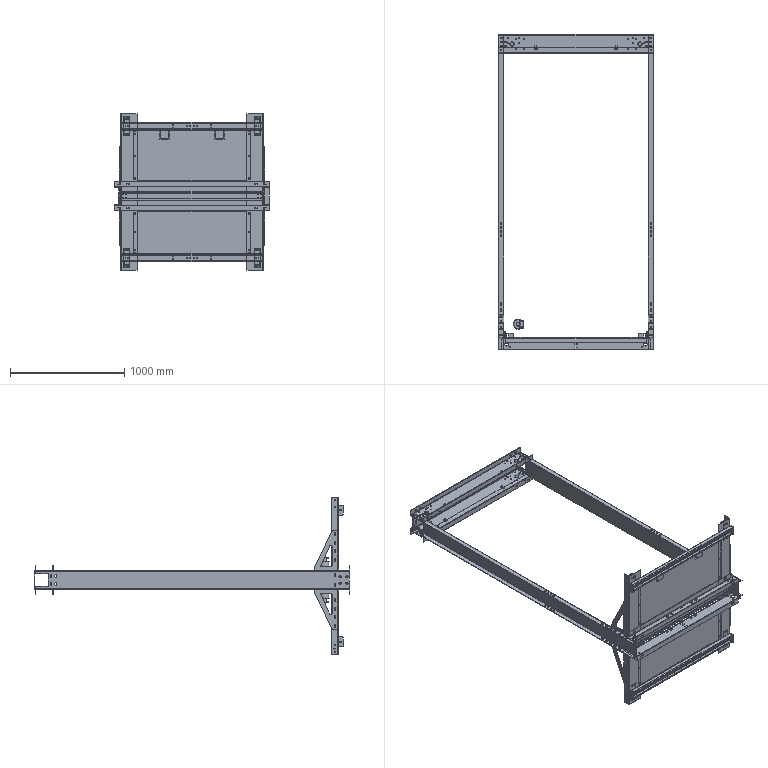Part | SolidWorks | features ReferencePattern 4, MirrorCompFeat 2 | 50 solids | 2544 faces | box 1350 x 2756 x 1370 mm | volume 24130984 mm3 | plane 1232 | cylinder 1184 | cone 124 | torus 4 | commonest cylinder face diameters 13 x260 14 x168 11 x116 7 x70 12 x70 6 x48